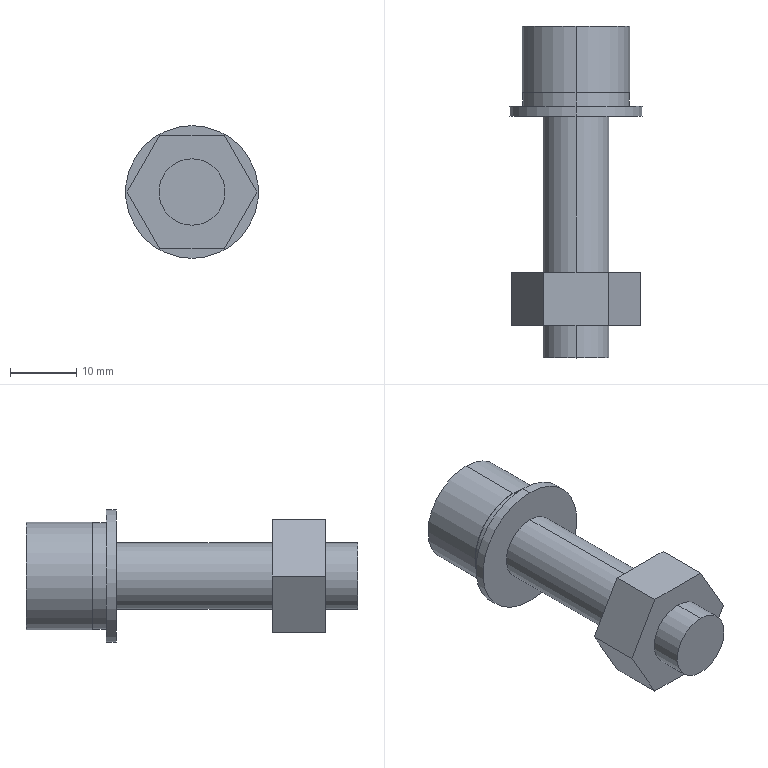Part | SolidWorks | features ICE 4, Revolution 1 | 3 solids | 36 faces | box 20 x 50 x 20 mm | volume 6831 mm3 | plane 22 | cylinder 14 | commonest cylinder face diameters 10 x8 16 x2 16.2 x2 20 x2
STEP:
#1=CARTESIAN_POINT('',(0.,-2.1,5.));
#2=VERTEX_POINT('',#1);
#3=CARTESIAN_POINT('',(0.,-2.1,-5.));
#4=VERTEX_POINT('',#3);
#5=CARTESIAN_POINT('',(0.,-2.1,0.));
#6=DIRECTION('',(0.,-1.,0.));
#7=DIRECTION('',(0.,0.,-1.));
#8=AXIS2_PLACEMENT_3D('',#5,#6,#7);
#9=CIRCLE('',#8,5.);
#10=EDGE_CURVE('',#2,#4,#9,.T.);
#11=ORIENTED_EDGE('',*,*,#10,.T.);
#12=CARTESIAN_POINT('',(0.,0.,-5.));
#13=VERTEX_POINT('',#12);
#14=CARTESIAN_POINT('',(0.,-2.1,-5.));
#15=DIRECTION('',(0.,1.,0.));
#16=VECTOR('',#15,1000.);
#17=LINE('',#14,#16);
#18=EDGE_CURVE('',#4,#13,#17,.T.);
#19=ORIENTED_EDGE('',*,*,#18,.T.);
#20=CARTESIAN_POINT('',(0.,0.,5.));
#21=VERTEX_POINT('',#20);
#22=CARTESIAN_POINT('',(0.,0.,0.));
#23=DIRECTION('',(0.,-1.,0.));
#24=DIRECTION('',(0.,0.,-1.));
#25=AXIS2_PLACEMENT_3D('',#22,#23,#24);
#26=CIRCLE('',#25,5.);
#27=EDGE_CURVE('',#21,#13,#26,.T.);
#28=ORIENTED_EDGE('',*,*,#27,.F.);
#29=CARTESIAN_POINT('',(0.,-2.1,5.));
#30=DIRECTION('',(0.,1.,0.));
#31=VECTOR('',#30,1000.);
#32=LINE('',#29,#31);
#33=EDGE_CURVE('',#2,#21,#32,.T.);
#34=ORIENTED_EDGE('',*,*,#33,.F.);
#35=EDGE_LOOP('',(#11,#19,#28,#34));
#36=FACE_OUTER_BOUND('',#35,.T.);
#37=CARTESIAN_POINT('',(0.,-2.1,0.));
#38=DIRECTION('',(0.,1.,0.));
#39=DIRECTION('',(0.,0.,1.));
#40=AXIS2_PLACEMENT_3D('',#37,#38,#39);
#41=CYLINDRICAL_SURFACE('',#40,5.);
#42=ADVANCED_FACE('',(#36),#41,.F.);
#43=CARTESIAN_POINT('',(0.,-2.1,-8.));
#44=VERTEX_POINT('',#43);
#45=CARTESIAN_POINT('',(0.,-2.1,8.));
#46=VERTEX_POINT('',#45);
#47=CARTESIAN_POINT('',(0.,-2.1,0.));
#48=DIRECTION('',(0.,-1.,0.));
#49=DIRECTION('',(0.,0.,-1.));
#50=AXIS2_PLACEMENT_3D('',#47,#48,#49);
#51=CIRCLE('',#50,8.);
#52=EDGE_CURVE('',#44,#46,#51,.T.);
#53=ORIENTED_EDGE('',*,*,#52,.F.);
#54=CARTESIAN_POINT('',(0.,0.,-8.));
#55=VERTEX_POINT('',#54);
#56=CARTESIAN_POINT('',(0.,-2.1,-8.));
#57=DIRECTION('',(0.,1.,0.));
#58=VECTOR('',#57,1000.);
#59=LINE('',#56,#58);
#60=EDGE_CURVE('',#44,#55,#59,.T.);
#61=ORIENTED_EDGE('',*,*,#60,.T.);
#62=CARTESIAN_POINT('',(0.,0.,8.));
#63=VERTEX_POINT('',#62);
#64=CARTESIAN_POINT('',(0.,0.,0.));
#65=DIRECTION('',(0.,-1.,0.));
#66=DIRECTION('',(0.,0.,-1.));
#67=AXIS2_PLACEMENT_3D('',#64,#65,#66);
#68=CIRCLE('',#67,8.);
#69=EDGE_CURVE('',#55,#63,#68,.T.);
#70=ORIENTED_EDGE('',*,*,#69,.T.);
#71=CARTESIAN_POINT('',(0.,-2.1,8.));
#72=DIRECTION('',(0.,1.,0.));
#73=VECTOR('',#72,1000.);
#74=LINE('',#71,#73);
#75=EDGE_CURVE('',#46,#63,#74,.T.);
#76=ORIENTED_EDGE('',*,*,#75,.F.);
#77=EDGE_LOOP('',(#53,#61,#70,#76));
#78=FACE_OUTER_BOUND('',#77,.T.);
#79=CARTESIAN_POINT('',(0.,-2.1,0.));
#80=DIRECTION('',(0.,1.,0.));
#81=DIRECTION('',(0.,0.,1.));
#82=AXIS2_PLACEMENT_3D('',#79,#80,#81);
#83=CYLINDRICAL_SURFACE('',#82,8.);
#84=ADVANCED_FACE('',(#78),#83,.T.);
#85=CARTESIAN_POINT('',(0.,-2.1,0.));
#86=DIRECTION('',(0.,-1.,0.));
#87=DIRECTION('',(0.,0.,-1.));
#88=AXIS2_PLACEMENT_3D('',#85,#86,#87);
#89=CIRCLE('',#88,8.);
#90=EDGE_CURVE('',#46,#44,#89,.T.);
#91=ORIENTED_EDGE('',*,*,#90,.T.);
#92=ORIENTED_EDGE('',*,*,#52,.T.);
#93=EDGE_LOOP('',(#91,#92));
#94=FACE_OUTER_BOUND('',#93,.T.);
#95=ORIENTED_EDGE('',*,*,#10,.F.);
#96=CARTESIAN_POINT('',(0.,-2.1,0.));
#97=DIRECTION('',(0.,-1.,0.));
#98=DIRECTION('',(0.,0.,-1.));
#99=AXIS2_PLACEMENT_3D('',#96,#97,#98);
#100=CIRCLE('',#99,5.);
#101=EDGE_CURVE('',#4,#2,#100,.T.);
#102=ORIENTED_EDGE('',*,*,#101,.F.);
#103=EDGE_LOOP('',(#95,#102));
#104=FACE_BOUND('',#103,.T.);
#105=CARTESIAN_POINT('',(0.,-2.1,0.));
#106=DIRECTION('',(0.,-1.,0.));
#107=DIRECTION('',(0.,0.,-1.));
#108=AXIS2_PLACEMENT_3D('',#105,#106,#107);
#109=PLANE('',#108);
#110=ADVANCED_FACE('',(#94,#104),#109,.T.);
#111=CARTESIAN_POINT('',(0.,0.,0.));
#112=DIRECTION('',(0.,-1.,0.));
#113=DIRECTION('',(0.,0.,-1.));
#114=AXIS2_PLACEMENT_3D('',#111,#112,#113);
#115=CIRCLE('',#114,8.);
#116=EDGE_CURVE('',#63,#55,#115,.T.);
#117=ORIENTED_EDGE('',*,*,#116,.F.);
#118=ORIENTED_EDGE('',*,*,#69,.F.);
#119=EDGE_LOOP('',(#117,#118));
#120=FACE_OUTER_BOUND('',#119,.T.);
#121=ORIENTED_EDGE('',*,*,#27,.T.);
#122=CARTESIAN_POINT('',(0.,0.,0.));
#123=DIRECTION('',(0.,-1.,0.));
#124=DIRECTION('',(0.,0.,-1.));
#125=AXIS2_PLACEMENT_3D('',#122,#123,#124);
#126=CIRCLE('',#125,5.);
#127=EDGE_CURVE('',#13,#21,#126,.T.);
#128=ORIENTED_EDGE('',*,*,#127,.T.);
#129=EDGE_LOOP('',(#121,#128));
#130=FACE_BOUND('',#129,.T.);
#131=CARTESIAN_POINT('',(0.,0.,0.));
#132=DIRECTION('',(0.,-1.,0.));
#133=DIRECTION('',(0.,0.,-1.));
#134=AXIS2_PLACEMENT_3D('',#131,#132,#133);
#135=PLANE('',#134);
#136=ADVANCED_FACE('',(#120,#130),#135,.F.);
#137=ORIENTED_EDGE('',*,*,#60,.F.);
#138=ORIENTED_EDGE('',*,*,#90,.F.);
#139=ORIENTED_EDGE('',*,*,#75,.T.);
#140=ORIENTED_EDGE('',*,*,#116,.T.);
#141=EDGE_LOOP('',(#137,#138,#139,#140));
#142=FACE_OUTER_BOUND('',#141,.T.);
#143=CARTESIAN_POINT('',(0.,-2.1,0.));
#144=DIRECTION('',(0.,1.,0.));
#145=DIRECTION('',(0.,0.,1.));
#146=AXIS2_PLACEMENT_3D('',#143,#144,#145);
#147=CYLINDRICAL_SURFACE('',#146,8.);
#148=ADVANCED_FACE('',(#142),#147,.T.);
#149=ORIENTED_EDGE('',*,*,#18,.F.);
#150=ORIENTED_EDGE('',*,*,#101,.T.);
#151=ORIENTED_EDGE('',*,*,#33,.T.);
#152=ORIENTED_EDGE('',*,*,#127,.F.);
#153=EDGE_LOOP('',(#149,#150,#151,#152));
#154=FACE_OUTER_BOUND('',#153,.T.);
#155=CARTESIAN_POINT('',(0.,-2.1,0.));
#156=DIRECTION('',(0.,1.,0.));
#157=DIRECTION('',(0.,0.,1.));
#158=AXIS2_PLACEMENT_3D('',#155,#156,#157);
#159=CYLINDRICAL_SURFACE('',#158,5.);
#160=ADVANCED_FACE('',(#154),#159,.F.);
#161=CLOSED_SHELL('',(#42,#84,#110,#136,#148,#160));
#162=MANIFOLD_SOLID_BREP('',#161);
#163=CARTESIAN_POINT('',(0.,-3.6,5.));
#164=VERTEX_POINT('',#163);
#165=CARTESIAN_POINT('',(0.,-3.6,-5.));
#166=VERTEX_POINT('',#165);
#167=CARTESIAN_POINT('',(0.,-3.6,0.));
#168=DIRECTION('',(0.,-1.,0.));
#169=DIRECTION('',(0.,0.,-1.));
#170=AXIS2_PLACEMENT_3D('',#167,#168,#169);
#171=CIRCLE('',#170,5.);
#172=EDGE_CURVE('',#164,#166,#171,.T.);
#173=ORIENTED_EDGE('',*,*,#172,.T.);
#174=CARTESIAN_POINT('',(0.,-2.1,-5.));
#175=VERTEX_POINT('',#174);
#176=CARTESIAN_POINT('',(0.,-3.6,-5.));
#177=DIRECTION('',(0.,1.,0.));
#178=VECTOR('',#177,1000.);
#179=LINE('',#176,#178);
#180=EDGE_CURVE('',#166,#175,#179,.T.);
#181=ORIENTED_EDGE('',*,*,#180,.T.);
#182=CARTESIAN_POINT('',(0.,-2.1,5.));
#183=VERTEX_POINT('',#182);
#184=CARTESIAN_POINT('',(0.,-2.1,0.));
#185=DIRECTION('',(0.,-1.,0.));
#186=DIRECTION('',(0.,0.,-1.));
#187=AXIS2_PLACEMENT_3D('',#184,#185,#186);
#188=CIRCLE('',#187,5.);
#189=EDGE_CURVE('',#183,#175,#188,.T.);
#190=ORIENTED_EDGE('',*,*,#189,.F.);
#191=CARTESIAN_POINT('',(0.,-3.6,5.));
#192=DIRECTION('',(0.,1.,0.));
#193=VECTOR('',#192,1000.);
#194=LINE('',#191,#193);
#195=EDGE_CURVE('',#164,#183,#194,.T.);
#196=ORIENTED_EDGE('',*,*,#195,.F.);
#197=EDGE_LOOP('',(#173,#181,#190,#196));
#198=FACE_OUTER_BOUND('',#197,.T.);
#199=CARTESIAN_POINT('',(0.,-3.6,0.));
#200=DIRECTION('',(0.,1.,0.));
#201=DIRECTION('',(0.,0.,1.));
#202=AXIS2_PLACEMENT_3D('',#199,#200,#201);
#203=CYLINDRICAL_SURFACE('',#202,5.);
#204=ADVANCED_FACE('',(#198),#203,.F.);
#205=CARTESIAN_POINT('',(0.,-3.6,-10.));
#206=VERTEX_POINT('',#205);
#207=CARTESIAN_POINT('',(0.,-3.6,10.));
#208=VERTEX_POINT('',#207);
#209=CARTESIAN_POINT('',(0.,-3.6,0.));
#210=DIRECTION('',(0.,-1.,0.));
#211=DIRECTION('',(0.,0.,-1.));
#212=AXIS2_PLACEMENT_3D('',#209,#210,#211);
#213=CIRCLE('',#212,10.);
#214=EDGE_CURVE('',#206,#208,#213,.T.);
#215=ORIENTED_EDGE('',*,*,#214,.F.);
#216=CARTESIAN_POINT('',(0.,-2.1,-10.));
#217=VERTEX_POINT('',#216);
#218=CARTESIAN_POINT('',(0.,-3.6,-10.));
#219=DIRECTION('',(0.,1.,0.));
#220=VECTOR('',#219,1000.);
#221=LINE('',#218,#220);
#222=EDGE_CURVE('',#206,#217,#221,.T.);
#223=ORIENTED_EDGE('',*,*,#222,.T.);
#224=CARTESIAN_POINT('',(0.,-2.1,10.));
#225=VERTEX_POINT('',#224);
#226=CARTESIAN_POINT('',(0.,-2.1,0.));
#227=DIRECTION('',(0.,-1.,0.));
#228=DIRECTION('',(0.,0.,-1.));
#229=AXIS2_PLACEMENT_3D('',#226,#227,#228);
#230=CIRCLE('',#229,10.);
#231=EDGE_CURVE('',#217,#225,#230,.T.);
#232=ORIENTED_EDGE('',*,*,#231,.T.);
#233=CARTESIAN_POINT('',(0.,-3.6,10.));
#234=DIRECTION('',(0.,1.,0.));
#235=VECTOR('',#234,1000.);
#236=LINE('',#233,#235);
#237=EDGE_CURVE('',#208,#225,#236,.T.);
#238=ORIENTED_EDGE('',*,*,#237,.F.);
#239=EDGE_LOOP('',(#215,#223,#232,#238));
#240=FACE_OUTER_BOUND('',#239,.T.);
#241=CARTESIAN_POINT('',(0.,-3.6,0.));
#242=DIRECTION('',(0.,1.,0.));
#243=DIRECTION('',(0.,0.,1.));
#244=AXIS2_PLACEMENT_3D('',#241,#242,#243);
#245=CYLINDRICAL_SURFACE('',#244,10.);
#246=ADVANCED_FACE('',(#240),#245,.T.);
#247=CARTESIAN_POINT('',(0.,-3.6,0.));
#248=DIRECTION('',(0.,-1.,0.));
#249=DIRECTION('',(0.,0.,-1.));
#250=AXIS2_PLACEMENT_3D('',#247,#248,#249);
#251=CIRCLE('',#250,10.);
#252=EDGE_CURVE('',#208,#206,#251,.T.);
#253=ORIENTED_EDGE('',*,*,#252,.T.);
#254=ORIENTED_EDGE('',*,*,#214,.T.);
#255=EDGE_LOOP('',(#253,#254));
#256=FACE_OUTER_BOUND('',#255,.T.);
#257=ORIENTED_EDGE('',*,*,#172,.F.);
#258=CARTESIAN_POINT('',(0.,-3.6,0.));
#259=DIRECTION('',(0.,-1.,0.));
#260=DIRECTION('',(0.,0.,-1.));
#261=AXIS2_PLACEMENT_3D('',#258,#259,#260);
#262=CIRCLE('',#261,5.);
#263=EDGE_CURVE('',#166,#164,#262,.T.);
#264=ORIENTED_EDGE('',*,*,#263,.F.);
#265=EDGE_LOOP('',(#257,#264));
#266=FACE_BOUND('',#265,.T.);
#267=CARTESIAN_POINT('',(0.,-3.6,0.));
#268=DIRECTION('',(0.,-1.,0.));
#269=DIRECTION('',(0.,0.,-1.));
#270=AXIS2_PLACEMENT_3D('',#267,#268,#269);
#271=PLANE('',#270);
#272=ADVANCED_FACE('',(#256,#266),#271,.T.);
#273=CARTESIAN_POINT('',(0.,-2.1,0.));
#274=DIRECTION('',(0.,-1.,0.));
#275=DIRECTION('',(0.,0.,-1.));
#276=AXIS2_PLACEMENT_3D('',#273,#274,#275);
#277=CIRCLE('',#276,10.);
#278=EDGE_CURVE('',#225,#217,#277,.T.);
#279=ORIENTED_EDGE('',*,*,#278,.F.);
#280=ORIENTED_EDGE('',*,*,#231,.F.);
#281=EDGE_LOOP('',(#279,#280));
#282=FACE_OUTER_BOUND('',#281,.T.);
#283=ORIENTED_EDGE('',*,*,#189,.T.);
#284=CARTESIAN_POINT('',(0.,-2.1,0.));
#285=DIRECTION('',(0.,-1.,0.));
#286=DIRECTION('',(0.,0.,-1.));
#287=AXIS2_PLACEMENT_3D('',#284,#285,#286);
#288=CIRCLE('',#287,5.);
#289=EDGE_CURVE('',#175,#183,#288,.T.);
#290=ORIENTED_EDGE('',*,*,#289,.T.);
#291=EDGE_LOOP('',(#283,#290));
#292=FACE_BOUND('',#291,.T.);
#293=CARTESIAN_POINT('',(0.,-2.1,0.));
#294=DIRECTION('',(0.,-1.,0.));
#295=DIRECTION('',(0.,0.,-1.));
#296=AXIS2_PLACEMENT_3D('',#293,#294,#295);
#297=PLANE('',#296);
#298=ADVANCED_FACE('',(#282,#292),#297,.F.);
#299=ORIENTED_EDGE('',*,*,#222,.F.);
#300=ORIENTED_EDGE('',*,*,#252,.F.);
#301=ORIENTED_EDGE('',*,*,#237,.T.);
#302=ORIENTED_EDGE('',*,*,#278,.T.);
#303=EDGE_LOOP('',(#299,#300,#301,#302));
#304=FACE_OUTER_BOUND('',#303,.T.);
#305=CARTESIAN_POINT('',(0.,-3.6,0.));
#306=DIRECTION('',(0.,1.,0.));
#307=DIRECTION('',(0.,0.,1.));
#308=AXIS2_PLACEMENT_3D('',#305,#306,#307);
#309=CYLINDRICAL_SURFACE('',#308,10.);
#310=ADVANCED_FACE('',(#304),#309,.T.);
#311=ORIENTED_EDGE('',*,*,#180,.F.);
#312=ORIENTED_EDGE('',*,*,#263,.T.);
#313=ORIENTED_EDGE('',*,*,#195,.T.);
#314=ORIENTED_EDGE('',*,*,#289,.F.);
#315=EDGE_LOOP('',(#311,#312,#313,#314));
#316=FACE_OUTER_BOUND('',#315,.T.);
#317=CARTESIAN_POINT('',(0.,-3.6,0.));
#318=DIRECTION('',(0.,1.,0.));
#319=DIRECTION('',(0.,0.,1.));
#320=AXIS2_PLACEMENT_3D('',#317,#318,#319);
#321=CYLINDRICAL_SURFACE('',#320,5.);
#322=ADVANCED_FACE('',(#316),#321,.F.);
#323=CLOSED_SHELL('',(#204,#246,#272,#298,#310,#322));
#324=MANIFOLD_SOLID_BREP('',#323);
#325=CARTESIAN_POINT('',(0.,-40.,5.));
#326=VERTEX_POINT('',#325);
#327=CARTESIAN_POINT('',(0.,-40.,-5.));
#328=VERTEX_POINT('',#327);
#329=CARTESIAN_POINT('',(0.,-40.,0.));
#330=DIRECTION('',(0.,1.,0.));
#331=DIRECTION('',(0.,0.,1.));
#332=AXIS2_PLACEMENT_3D('',#329,#330,#331);
#333=CIRCLE('',#332,5.);
#334=EDGE_CURVE('',#326,#328,#333,.T.);
#335=ORIENTED_EDGE('',*,*,#334,.T.);
#336=CARTESIAN_POINT('',(0.,-35.1,-5.));
#337=VERTEX_POINT('',#336);
#338=CARTESIAN_POINT('',(0.,11.322,-5.));
#339=DIRECTION('',(0.,1.,0.));
#340=VECTOR('',#339,1000.);
#341=LINE('',#338,#340);
#342=EDGE_CURVE('',#328,#337,#341,.T.);
#343=ORIENTED_EDGE('',*,*,#342,.T.);
#344=CARTESIAN_POINT('',(0.,-35.1,5.));
#345=VERTEX_POINT('',#344);
#346=CARTESIAN_POINT('',(0.,-35.1,0.));
#347=DIRECTION('',(0.,1.,0.));
#348=DIRECTION('',(0.,0.,-1.));
#349=AXIS2_PLACEMENT_3D('',#346,#347,#348);
#350=CIRCLE('',#349,5.);
#351=EDGE_CURVE('',#345,#337,#350,.T.);
#352=ORIENTED_EDGE('',*,*,#351,.F.);
#353=CARTESIAN_POINT('',(0.,11.322,5.));
#354=DIRECTION('',(0.,1.,0.));
#355=VECTOR('',#354,1000.);
#356=LINE('',#353,#355);
#357=EDGE_CURVE('',#326,#345,#356,.T.);
#358=ORIENTED_EDGE('',*,*,#357,.F.);
#359=EDGE_LOOP('',(#335,#343,#352,#358));
#360=FACE_OUTER_BOUND('',#359,.T.);
#361=CARTESIAN_POINT('',(0.,11.322,0.));
#362=DIRECTION('',(0.,1.,0.));
#363=DIRECTION('',(0.,0.,1.));
#364=AXIS2_PLACEMENT_3D('',#361,#362,#363);
#365=CYLINDRICAL_SURFACE('',#364,5.);
#366=ADVANCED_FACE('',(#360),#365,.T.);
#367=CARTESIAN_POINT('',(0.,0.,8.1));
#368=VERTEX_POINT('',#367);
#369=CARTESIAN_POINT('',(0.,0.,-8.1));
#370=VERTEX_POINT('',#369);
#371=CARTESIAN_POINT('',(0.,0.,0.));
#372=DIRECTION('',(0.,1.,0.));
#373=DIRECTION('',(0.,0.,1.));
#374=AXIS2_PLACEMENT_3D('',#371,#372,#373);
#375=CIRCLE('',#374,8.1);
#376=EDGE_CURVE('',#368,#370,#375,.T.);
#377=ORIENTED_EDGE('',*,*,#376,.T.);
#378=CARTESIAN_POINT('',(0.,10.,-8.1));
#379=VERTEX_POINT('',#378);
#380=CARTESIAN_POINT('',(0.,11.322,-8.1));
#381=DIRECTION('',(0.,1.,0.));
#382=VECTOR('',#381,1000.);
#383=LINE('',#380,#382);
#384=EDGE_CURVE('',#370,#379,#383,.T.);
#385=ORIENTED_EDGE('',*,*,#384,.T.);
#386=CARTESIAN_POINT('',(0.,10.,8.1));
#387=VERTEX_POINT('',#386);
#388=CARTESIAN_POINT('',(0.,10.,0.));
#389=DIRECTION('',(0.,1.,0.));
#390=DIRECTION('',(0.,0.,1.));
#391=AXIS2_PLACEMENT_3D('',#388,#389,#390);
#392=CIRCLE('',#391,8.1);
#393=EDGE_CURVE('',#387,#379,#392,.T.);
#394=ORIENTED_EDGE('',*,*,#393,.F.);
#395=CARTESIAN_POINT('',(0.,11.322,8.1));
#396=DIRECTION('',(0.,1.,0.));
#397=VECTOR('',#396,1000.);
#398=LINE('',#395,#397);
#399=EDGE_CURVE('',#368,#387,#398,.T.);
#400=ORIENTED_EDGE('',*,*,#399,.F.);
#401=EDGE_LOOP('',(#377,#385,#394,#400));
#402=FACE_OUTER_BOUND('',#401,.T.);
#403=CARTESIAN_POINT('',(0.,11.322,0.));
#404=DIRECTION('',(0.,1.,0.));
#405=DIRECTION('',(0.,0.,1.));
#406=AXIS2_PLACEMENT_3D('',#403,#404,#405);
#407=CYLINDRICAL_SURFACE('',#406,8.1);
#408=ADVANCED_FACE('',(#402),#407,.T.);
#409=CARTESIAN_POINT('',(0.,-27.1,-5.));
#410=VERTEX_POINT('',#409);
#411=CARTESIAN_POINT('',(0.,-27.1,5.));
#412=VERTEX_POINT('',#411);
#413=CARTESIAN_POINT('',(0.,-27.1,0.));
#414=DIRECTION('',(0.,-1.,0.));
#415=DIRECTION('',(0.,0.,-1.));
#416=AXIS2_PLACEMENT_3D('',#413,#414,#415);
#417=CIRCLE('',#416,5.);
#418=EDGE_CURVE('',#410,#412,#417,.T.);
#419=ORIENTED_EDGE('',*,*,#418,.F.);
#420=CARTESIAN_POINT('',(0.,0.,-5.));
#421=VERTEX_POINT('',#420);
#422=CARTESIAN_POINT('',(0.,11.322,-5.));
#423=DIRECTION('',(0.,1.,0.));
#424=VECTOR('',#423,1000.);
#425=LINE('',#422,#424);
#426=EDGE_CURVE('',#410,#421,#425,.T.);
#427=ORIENTED_EDGE('',*,*,#426,.T.);
#428=CARTESIAN_POINT('',(0.,0.,5.));
#429=VERTEX_POINT('',#428);
#430=CARTESIAN_POINT('',(0.,0.,0.));
#431=DIRECTION('',(0.,1.,0.));
#432=DIRECTION('',(0.,0.,1.));
#433=AXIS2_PLACEMENT_3D('',#430,#431,#432);
#434=CIRCLE('',#433,5.);
#435=EDGE_CURVE('',#429,#421,#434,.T.);
#436=ORIENTED_EDGE('',*,*,#435,.F.);
#437=CARTESIAN_POINT('',(0.,11.322,5.));
#438=DIRECTION('',(0.,1.,0.));
#439=VECTOR('',#438,1000.);
#440=LINE('',#437,#439);
#441=EDGE_CURVE('',#412,#429,#440,.T.);
#442=ORIENTED_EDGE('',*,*,#441,.F.);
#443=EDGE_LOOP('',(#419,#427,#436,#442));
#444=FACE_OUTER_BOUND('',#443,.T.);
#445=CARTESIAN_POINT('',(0.,11.322,0.));
#446=DIRECTION('',(0.,1.,0.));
#447=DIRECTION('',(0.,0.,1.));
#448=AXIS2_PLACEMENT_3D('',#445,#446,#447);
#449=CYLINDRICAL_SURFACE('',#448,5.);
#450=ADVANCED_FACE('',(#444),#449,.T.);
#451=ORIENTED_EDGE('',*,*,#426,.F.);
#452=CARTESIAN_POINT('',(0.,-27.1,0.));
#453=DIRECTION('',(0.,-1.,0.));
#454=DIRECTION('',(0.,0.,-1.));
#455=AXIS2_PLACEMENT_3D('',#452,#453,#454);
#456=CIRCLE('',#455,5.);
#457=EDGE_CURVE('',#412,#410,#456,.T.);
#458=ORIENTED_EDGE('',*,*,#457,.F.);
#459=ORIENTED_EDGE('',*,*,#441,.T.);
#460=CARTESIAN_POINT('',(0.,0.,0.));
#461=DIRECTION('',(0.,1.,0.));
#462=DIRECTION('',(0.,0.,1.));
#463=AXIS2_PLACEMENT_3D('',#460,#461,#462);
#464=CIRCLE('',#463,5.);
#465=EDGE_CURVE('',#421,#429,#464,.T.);
#466=ORIENTED_EDGE('',*,*,#465,.F.);
#467=EDGE_LOOP('',(#451,#458,#459,#466));
#468=FACE_OUTER_BOUND('',#467,.T.);
#469=CARTESIAN_POINT('',(0.,11.322,0.));
#470=DIRECTION('',(0.,1.,0.));
#471=DIRECTION('',(0.,0.,1.));
#472=AXIS2_PLACEMENT_3D('',#469,#470,#471);
#473=CYLINDRICAL_SURFACE('',#472,5.);
#474=ADVANCED_FACE('',(#468),#473,.T.);
#475=CARTESIAN_POINT('',(4.,10.,-2.309));
#476=VERTEX_POINT('',#475);
#477=CARTESIAN_POINT('',(0.,10.,-4.619));
#478=VERTEX_POINT('',#477);
#479=CARTESIAN_POINT('',(4.,10.,-2.309));
#480=DIRECTION('',(-0.866,0.,-0.5));
#481=VECTOR('',#480,1000.);
#482=LINE('',#479,#481);
#483=EDGE_CURVE('',#476,#478,#482,.T.);
#484=ORIENTED_EDGE('',*,*,#483,.F.);
#485=CARTESIAN_POINT('',(4.,10.,2.309));
#486=VERTEX_POINT('',#485);
#487=CARTESIAN_POINT('',(4.,10.,2.309));
#488=DIRECTION('',(0.,0.,-1.));
#489=VECTOR('',#488,1000.);
#490=LINE('',#487,#489);
#491=EDGE_CURVE('',#486,#476,#490,.T.);
#492=ORIENTED_EDGE('',*,*,#491,.F.);
#493=CARTESIAN_POINT('',(0.,10.,4.619));
#494=VERTEX_POINT('',#493);
#495=CARTESIAN_POINT('',(0.,10.,4.619));
#496=DIRECTION('',(0.866,0.,-0.5));
#497=VECTOR('',#496,1000.);
#498=LINE('',#495,#497);
#499=EDGE_CURVE('',#494,#486,#498,.T.);
#500=ORIENTED_EDGE('',*,*,#499,.F.);
#501=CARTESIAN_POINT('',(-4.,10.,2.309));
#502=VERTEX_POINT('',#501);
#503=CARTESIAN_POINT('',(-4.,10.,2.309));
#504=DIRECTION('',(0.866,0.,0.5));
#505=VECTOR('',#504,1000.);
#506=LINE('',#503,#505);
#507=EDGE_CURVE('',#502,#494,#506,.T.);
#508=ORIENTED_EDGE('',*,*,#507,.F.);
#509=CARTESIAN_POINT('',(-4.,10.,-2.309));
#510=VERTEX_POINT('',#509);
#511=CARTESIAN_POINT('',(-4.,10.,-2.309));
#512=DIRECTION('',(0.,0.,1.));
#513=VECTOR('',#512,1000.);
#514=LINE('',#511,#513);
#515=EDGE_CURVE('',#510,#502,#514,.T.);
#516=ORIENTED_EDGE('',*,*,#515,.F.);
#517=CARTESIAN_POINT('',(0.,10.,-4.619));
#518=DIRECTION('',(-0.866,0.,0.5));
#519=VECTOR('',#518,1000.);
#520=LINE('',#517,#519);
#521=EDGE_CURVE('',#478,#510,#520,.T.);
#522=ORIENTED_EDGE('',*,*,#521,.F.);
#523=EDGE_LOOP('',(#484,#492,#500,#508,#516,#522));
#524=FACE_BOUND('',#523,.T.);
#525=ORIENTED_EDGE('',*,*,#393,.T.);
#526=CARTESIAN_POINT('',(0.,10.,0.));
#527=DIRECTION('',(0.,1.,0.));
#528=DIRECTION('',(0.,0.,1.));
#529=AXIS2_PLACEMENT_3D('',#526,#527,#528);
#530=CIRCLE('',#529,8.1);
#531=EDGE_CURVE('',#379,#387,#530,.T.);
#532=ORIENTED_EDGE('',*,*,#531,.T.);
#533=EDGE_LOOP('',(#525,#532));
#534=FACE_OUTER_BOUND('',#533,.T.);
#535=CARTESIAN_POINT('',(0.,10.,0.));
#536=DIRECTION('',(0.,1.,0.));
#537=DIRECTION('',(0.,0.,1.));
#538=AXIS2_PLACEMENT_3D('',#535,#536,#537);
#539=PLANE('',#538);
#540=ADVANCED_FACE('',(#524,#534),#539,.T.);
#541=ORIENTED_EDGE('',*,*,#384,.F.);
#542=CARTESIAN_POINT('',(0.,0.,0.));
#543=DIRECTION('',(0.,1.,0.));
#544=DIRECTION('',(0.,0.,1.));
#545=AXIS2_PLACEMENT_3D('',#542,#543,#544);
#546=CIRCLE('',#545,8.1);
#547=EDGE_CURVE('',#370,#368,#546,.T.);
#548=ORIENTED_EDGE('',*,*,#547,.T.);
#549=ORIENTED_EDGE('',*,*,#399,.T.);
#550=ORIENTED_EDGE('',*,*,#531,.F.);
#551=EDGE_LOOP('',(#541,#548,#549,#550));
#552=FACE_OUTER_BOUND('',#551,.T.);
#553=CARTESIAN_POINT('',(0.,11.322,0.));
#554=DIRECTION('',(0.,1.,0.));
#555=DIRECTION('',(0.,0.,1.));
#556=AXIS2_PLACEMENT_3D('',#553,#554,#555);
#557=CYLINDRICAL_SURFACE('',#556,8.1);
#558=ADVANCED_FACE('',(#552),#557,.T.);
#559=ORIENTED_EDGE('',*,*,#435,.T.);
#560=ORIENTED_EDGE('',*,*,#465,.T.);
#561=EDGE_LOOP('',(#559,#560));
#562=FACE_BOUND('',#561,.T.);
#563=ORIENTED_EDGE('',*,*,#376,.F.);
#564=ORIENTED_EDGE('',*,*,#547,.F.);
#565=EDGE_LOOP('',(#563,#564));
#566=FACE_OUTER_BOUND('',#565,.T.);
#567=CARTESIAN_POINT('',(-8.1,0.,0.));
#568=DIRECTION('',(0.,-1.,0.));
#569=DIRECTION('',(0.,0.,-1.));
#570=AXIS2_PLACEMENT_3D('',#567,#568,#569);
#571=PLANE('',#570);
#572=ADVANCED_FACE('',(#562,#566),#571,.T.);
#573=ORIENTED_EDGE('',*,*,#483,.T.);
#574=CARTESIAN_POINT('',(0.,4.,-4.619));
#575=VERTEX_POINT('',#574);
#576=CARTESIAN_POINT('',(0.,4.,-4.619));
#577=DIRECTION('',(0.,1.,0.));
#578=VECTOR('',#577,1000.);
#579=LINE('',#576,#578);
#580=EDGE_CURVE('',#575,#478,#579,.T.);
#581=ORIENTED_EDGE('',*,*,#580,.F.);
#582=CARTESIAN_POINT('',(4.,4.,-2.309));
#583=VERTEX_POINT('',#582);
#584=CARTESIAN_POINT('',(4.,4.,-2.309));
#585=DIRECTION('',(-0.866,0.,-0.5));
#586=VECTOR('',#585,1000.);
#587=LINE('',#584,#586);
#588=EDGE_CURVE('',#583,#575,#587,.T.);
#589=ORIENTED_EDGE('',*,*,#588,.F.);
#590=CARTESIAN_POINT('',(4.,4.,-2.309));
#591=DIRECTION('',(0.,1.,0.));
#592=VECTOR('',#591,1000.);
#593=LINE('',#590,#592);
#594=EDGE_CURVE('',#583,#476,#593,.T.);
#595=ORIENTED_EDGE('',*,*,#594,.T.);
#596=EDGE_LOOP('',(#573,#581,#589,#595));
#597=FACE_OUTER_BOUND('',#596,.T.);
#598=CARTESIAN_POINT('',(4.,4.,-2.309));
#599=DIRECTION('',(0.5,0.,-0.866));
#600=DIRECTION('',(-0.866,0.,-0.5));
#601=AXIS2_PLACEMENT_3D('',#598,#599,#600);
#602=PLANE('',#601);
#603=ADVANCED_FACE('',(#597),#602,.F.);
#604=ORIENTED_EDGE('',*,*,#491,.T.);
#605=ORIENTED_EDGE('',*,*,#594,.F.);
#606=CARTESIAN_POINT('',(4.,4.,2.309));
#607=VERTEX_POINT('',#606);
#608=CARTESIAN_POINT('',(4.,4.,2.309));
#609=DIRECTION('',(0.,0.,-1.));
#610=VECTOR('',#609,1000.);
#611=LINE('',#608,#610);
#612=EDGE_CURVE('',#607,#583,#611,.T.);
#613=ORIENTED_EDGE('',*,*,#612,.F.);
#614=CARTESIAN_POINT('',(4.,4.,2.309));
#615=DIRECTION('',(0.,1.,0.));
#616=VECTOR('',#615,1000.);
#617=LINE('',#614,#616);
#618=EDGE_CURVE('',#607,#486,#617,.T.);
#619=ORIENTED_EDGE('',*,*,#618,.T.);
#620=EDGE_LOOP('',(#604,#605,#613,#619));
#621=FACE_OUTER_BOUND('',#620,.T.);
#622=CARTESIAN_POINT('',(4.,4.,2.309));
#623=DIRECTION('',(1.,0.,0.));
#624=DIRECTION('',(0.,0.,-1.));
#625=AXIS2_PLACEMENT_3D('',#622,#623,#624);
#626=PLANE('',#625);
#627=ADVANCED_FACE('',(#621),#626,.F.);
#628=ORIENTED_EDGE('',*,*,#499,.T.);
#629=ORIENTED_EDGE('',*,*,#618,.F.);
#630=CARTESIAN_POINT('',(0.,4.,4.619));
#631=VERTEX_POINT('',#630);
#632=CARTESIAN_POINT('',(0.,4.,4.619));
#633=DIRECTION('',(0.866,0.,-0.5));
#634=VECTOR('',#633,1000.);
#635=LINE('',#632,#634);
#636=EDGE_CURVE('',#631,#607,#635,.T.);
#637=ORIENTED_EDGE('',*,*,#636,.F.);
#638=CARTESIAN_POINT('',(0.,4.,4.619));
#639=DIRECTION('',(0.,1.,0.));
#640=VECTOR('',#639,1000.);
#641=LINE('',#638,#640);
#642=EDGE_CURVE('',#631,#494,#641,.T.);
#643=ORIENTED_EDGE('',*,*,#642,.T.);
#644=EDGE_LOOP('',(#628,#629,#637,#643));
#645=FACE_OUTER_BOUND('',#644,.T.);
#646=CARTESIAN_POINT('',(0.,4.,4.619));
#647=DIRECTION('',(0.5,0.,0.866));
#648=DIRECTION('',(0.866,0.,-0.5));
#649=AXIS2_PLACEMENT_3D('',#646,#647,#648);
#650=PLANE('',#649);
#651=ADVANCED_FACE('',(#645),#650,.F.);
#652=ORIENTED_EDGE('',*,*,#507,.T.);
#653=ORIENTED_EDGE('',*,*,#642,.F.);
#654=CARTESIAN_POINT('',(-4.,4.,2.309));
#655=VERTEX_POINT('',#654);
#656=CARTESIAN_POINT('',(-4.,4.,2.309));
#657=DIRECTION('',(0.866,0.,0.5));
#658=VECTOR('',#657,1000.);
#659=LINE('',#656,#658);
#660=EDGE_CURVE('',#655,#631,#659,.T.);
#661=ORIENTED_EDGE('',*,*,#660,.F.);
#662=CARTESIAN_POINT('',(-4.,4.,2.309));
#663=DIRECTION('',(0.,1.,0.));
#664=VECTOR('',#663,1000.);
#665=LINE('',#662,#664);
#666=EDGE_CURVE('',#655,#502,#665,.T.);
#667=ORIENTED_EDGE('',*,*,#666,.T.);
#668=EDGE_LOOP('',(#652,#653,#661,#667));
#669=FACE_OUTER_BOUND('',#668,.T.);
#670=CARTESIAN_POINT('',(-4.,4.,2.309));
#671=DIRECTION('',(-0.5,0.,0.866));
#672=DIRECTION('',(0.866,0.,0.5));
#673=AXIS2_PLACEMENT_3D('',#670,#671,#672);
#674=PLANE('',#673);
#675=ADVANCED_FACE('',(#669),#674,.F.);
#676=ORIENTED_EDGE('',*,*,#515,.T.);
#677=ORIENTED_EDGE('',*,*,#666,.F.);
#678=CARTESIAN_POINT('',(-4.,4.,-2.309));
#679=VERTEX_POINT('',#678);
#680=CARTESIAN_POINT('',(-4.,4.,-2.309));
#681=DIRECTION('',(0.,0.,1.));
#682=VECTOR('',#681,1000.);
#683=LINE('',#680,#682);
#684=EDGE_CURVE('',#679,#655,#683,.T.);
#685=ORIENTED_EDGE('',*,*,#684,.F.);
#686=CARTESIAN_POINT('',(-4.,4.,-2.309));
#687=DIRECTION('',(0.,1.,0.));
#688=VECTOR('',#687,1000.);
#689=LINE('',#686,#688);
#690=EDGE_CURVE('',#679,#510,#689,.T.);
#691=ORIENTED_EDGE('',*,*,#690,.T.);
#692=EDGE_LOOP('',(#676,#677,#685,#691));
#693=FACE_OUTER_BOUND('',#692,.T.);
#694=CARTESIAN_POINT('',(-4.,4.,-2.309));
#695=DIRECTION('',(-1.,0.,0.));
#696=DIRECTION('',(0.,0.,1.));
#697=AXIS2_PLACEMENT_3D('',#694,#695,#696);
#698=PLANE('',#697);
#699=ADVANCED_FACE('',(#693),#698,.F.);
#700=ORIENTED_EDGE('',*,*,#521,.T.);
#701=ORIENTED_EDGE('',*,*,#690,.F.);
#702=CARTESIAN_POINT('',(0.,4.,-4.619));
#703=DIRECTION('',(-0.866,0.,0.5));
#704=VECTOR('',#703,1000.);
#705=LINE('',#702,#704);
#706=EDGE_CURVE('',#575,#679,#705,.T.);
#707=ORIENTED_EDGE('',*,*,#706,.F.);
#708=ORIENTED_EDGE('',*,*,#580,.T.);
#709=EDGE_LOOP('',(#700,#701,#707,#708));
#710=FACE_OUTER_BOUND('',#709,.T.);
#711=CARTESIAN_POINT('',(0.,4.,-4.619));
#712=DIRECTION('',(-0.5,0.,-0.866));
#713=DIRECTION('',(-0.866,0.,0.5));
#714=AXIS2_PLACEMENT_3D('',#711,#712,#713);
#715=PLANE('',#714);
#716=ADVANCED_FACE('',(#710),#715,.F.);
#717=ORIENTED_EDGE('',*,*,#588,.T.);
#718=ORIENTED_EDGE('',*,*,#706,.T.);
#719=ORIENTED_EDGE('',*,*,#684,.T.);
#720=ORIENTED_EDGE('',*,*,#660,.T.);
#721=ORIENTED_EDGE('',*,*,#636,.T.);
#722=ORIENTED_EDGE('',*,*,#612,.T.);
#723=EDGE_LOOP('',(#717,#718,#719,#720,#721,#722));
#724=FACE_OUTER_BOUND('',#723,.T.);
#725=CARTESIAN_POINT('',(0.,4.,0.));
#726=DIRECTION('',(0.,1.,0.));
#727=DIRECTION('',(0.,0.,1.));
#728=AXIS2_PLACEMENT_3D('',#725,#726,#727);
#729=PLANE('',#728);
#730=ADVANCED_FACE('',(#724),#729,.T.);
#731=CARTESIAN_POINT('',(4.879,-35.1,-8.45));
#732=VERTEX_POINT('',#731);
#733=CARTESIAN_POINT('',(9.757,-35.1,0.));
#734=VERTEX_POINT('',#733);
#735=CARTESIAN_POINT('',(4.879,-35.1,-8.45));
#736=DIRECTION('',(0.5,0.,0.866));
#737=VECTOR('',#736,1000.);
#738=LINE('',#735,#737);
#739=EDGE_CURVE('',#732,#734,#738,.T.);
#740=ORIENTED_EDGE('',*,*,#739,.T.);
#741=CARTESIAN_POINT('',(4.879,-35.1,8.45));
#742=VERTEX_POINT('',#741);
#743=CARTESIAN_POINT('',(9.757,-35.1,0.));
#744=DIRECTION('',(-0.5,0.,0.866));
#745=VECTOR('',#744,1000.);
#746=LINE('',#743,#745);
#747=EDGE_CURVE('',#734,#742,#746,.T.);
#748=ORIENTED_EDGE('',*,*,#747,.T.);
#749=CARTESIAN_POINT('',(-4.879,-35.1,8.45));
#750=VERTEX_POINT('',#749);
#751=CARTESIAN_POINT('',(4.879,-35.1,8.45));
#752=DIRECTION('',(-1.,0.,0.));
#753=VECTOR('',#752,1000.);
#754=LINE('',#751,#753);
#755=EDGE_CURVE('',#742,#750,#754,.T.);
#756=ORIENTED_EDGE('',*,*,#755,.T.);
#757=CARTESIAN_POINT('',(-9.757,-35.1,0.));
#758=VERTEX_POINT('',#757);
#759=CARTESIAN_POINT('',(-4.879,-35.1,8.45));
#760=DIRECTION('',(-0.5,0.,-0.866));
#761=VECTOR('',#760,1000.);
#762=LINE('',#759,#761);
#763=EDGE_CURVE('',#750,#758,#762,.T.);
#764=ORIENTED_EDGE('',*,*,#763,.T.);
#765=CARTESIAN_POINT('',(-4.879,-35.1,-8.45));
#766=VERTEX_POINT('',#765);
#767=CARTESIAN_POINT('',(-9.757,-35.1,0.));
#768=DIRECTION('',(0.5,0.,-0.866));
#769=VECTOR('',#768,1000.);
#770=LINE('',#767,#769);
#771=EDGE_CURVE('',#758,#766,#770,.T.);
#772=ORIENTED_EDGE('',*,*,#771,.T.);
#773=CARTESIAN_POINT('',(-4.879,-35.1,-8.45));
#774=DIRECTION('',(1.,0.,0.));
#775=VECTOR('',#774,1000.);
#776=LINE('',#773,#775);
#777=EDGE_CURVE('',#766,#732,#776,.T.);
#778=ORIENTED_EDGE('',*,*,#777,.T.);
#779=EDGE_LOOP('',(#740,#748,#756,#764,#772,#778));
#780=FACE_OUTER_BOUND('',#779,.T.);
#781=ORIENTED_EDGE('',*,*,#351,.T.);
#782=CARTESIAN_POINT('',(0.,-35.1,0.));
#783=DIRECTION('',(0.,1.,0.));
#784=DIRECTION('',(0.,0.,-1.));
#785=AXIS2_PLACEMENT_3D('',#782,#783,#784);
#786=CIRCLE('',#785,5.);
#787=EDGE_CURVE('',#337,#345,#786,.T.);
#788=ORIENTED_EDGE('',*,*,#787,.T.);
#789=EDGE_LOOP('',(#781,#788));
#790=FACE_BOUND('',#789,.T.);
#791=CARTESIAN_POINT('',(0.,-35.1,0.));
#792=DIRECTION('',(0.,-1.,0.));
#793=DIRECTION('',(0.,0.,-1.));
#794=AXIS2_PLACEMENT_3D('',#791,#792,#793);
#795=PLANE('',#794);
#796=ADVANCED_FACE('',(#780,#790),#795,.T.);
#797=CARTESIAN_POINT('',(4.879,-27.1,-8.45));
#798=VERTEX_POINT('',#797);
#799=CARTESIAN_POINT('',(9.757,-27.1,0.));
#800=VERTEX_POINT('',#799);
#801=CARTESIAN_POINT('',(4.879,-27.1,-8.45));
#802=DIRECTION('',(0.5,0.,0.866));
#803=VECTOR('',#802,1000.);
#804=LINE('',#801,#803);
#805=EDGE_CURVE('',#798,#800,#804,.T.);
#806=ORIENTED_EDGE('',*,*,#805,.F.);
#807=CARTESIAN_POINT('',(-4.879,-27.1,-8.45));
#808=VERTEX_POINT('',#807);
#809=CARTESIAN_POINT('',(-4.879,-27.1,-8.45));
#810=DIRECTION('',(1.,0.,0.));
#811=VECTOR('',#810,1000.);
#812=LINE('',#809,#811);
#813=EDGE_CURVE('',#808,#798,#812,.T.);
#814=ORIENTED_EDGE('',*,*,#813,.F.);
#815=CARTESIAN_POINT('',(-9.757,-27.1,0.));
#816=VERTEX_POINT('',#815);
#817=CARTESIAN_POINT('',(-9.757,-27.1,0.));
#818=DIRECTION('',(0.5,0.,-0.866));
#819=VECTOR('',#818,1000.);
#820=LINE('',#817,#819);
#821=EDGE_CURVE('',#816,#808,#820,.T.);
#822=ORIENTED_EDGE('',*,*,#821,.F.);
#823=CARTESIAN_POINT('',(-4.879,-27.1,8.45));
#824=VERTEX_POINT('',#823);
#825=CARTESIAN_POINT('',(-4.879,-27.1,8.45));
#826=DIRECTION('',(-0.5,0.,-0.866));
#827=VECTOR('',#826,1000.);
#828=LINE('',#825,#827);
#829=EDGE_CURVE('',#824,#816,#828,.T.);
#830=ORIENTED_EDGE('',*,*,#829,.F.);
#831=CARTESIAN_POINT('',(4.879,-27.1,8.45));
#832=VERTEX_POINT('',#831);
#833=CARTESIAN_POINT('',(4.879,-27.1,8.45));
#834=DIRECTION('',(-1.,0.,0.));
#835=VECTOR('',#834,1000.);
#836=LINE('',#833,#835);
#837=EDGE_CURVE('',#832,#824,#836,.T.);
#838=ORIENTED_EDGE('',*,*,#837,.F.);
#839=CARTESIAN_POINT('',(9.757,-27.1,0.));
#840=DIRECTION('',(-0.5,0.,0.866));
#841=VECTOR('',#840,1000.);
#842=LINE('',#839,#841);
#843=EDGE_CURVE('',#800,#832,#842,.T.);
#844=ORIENTED_EDGE('',*,*,#843,.F.);
#845=EDGE_LOOP('',(#806,#814,#822,#830,#838,#844));
#846=FACE_OUTER_BOUND('',#845,.T.);
#847=ORIENTED_EDGE('',*,*,#457,.T.);
#848=ORIENTED_EDGE('',*,*,#418,.T.);
#849=EDGE_LOOP('',(#847,#848));
#850=FACE_BOUND('',#849,.T.);
#851=CARTESIAN_POINT('',(0.,-27.1,0.));
#852=DIRECTION('',(0.,-1.,0.));
#853=DIRECTION('',(0.,0.,-1.));
#854=AXIS2_PLACEMENT_3D('',#851,#852,#853);
#855=PLANE('',#854);
#856=ADVANCED_FACE('',(#846,#850),#855,.F.);
#857=ORIENTED_EDGE('',*,*,#805,.T.);
#858=CARTESIAN_POINT('',(9.757,-35.1,0.));
#859=DIRECTION('',(0.,1.,0.));
#860=VECTOR('',#859,1000.);
#861=LINE('',#858,#860);
#862=EDGE_CURVE('',#734,#800,#861,.T.);
#863=ORIENTED_EDGE('',*,*,#862,.F.);
#864=ORIENTED_EDGE('',*,*,#739,.F.);
#865=CARTESIAN_POINT('',(4.879,-35.1,-8.45));
#866=DIRECTION('',(0.,1.,0.));
#867=VECTOR('',#866,1000.);
#868=LINE('',#865,#867);
#869=EDGE_CURVE('',#732,#798,#868,.T.);
#870=ORIENTED_EDGE('',*,*,#869,.T.);
#871=EDGE_LOOP('',(#857,#863,#864,#870));
#872=FACE_OUTER_BOUND('',#871,.T.);
#873=CARTESIAN_POINT('',(4.879,-35.1,-8.45));
#874=DIRECTION('',(-0.866,0.,0.5));
#875=DIRECTION('',(0.5,0.,0.866));
#876=AXIS2_PLACEMENT_3D('',#873,#874,#875);
#877=PLANE('',#876);
#878=ADVANCED_FACE('',(#872),#877,.F.);
#879=ORIENTED_EDGE('',*,*,#843,.T.);
#880=CARTESIAN_POINT('',(4.879,-35.1,8.45));
#881=DIRECTION('',(0.,1.,0.));
#882=VECTOR('',#881,1000.);
#883=LINE('',#880,#882);
#884=EDGE_CURVE('',#742,#832,#883,.T.);
#885=ORIENTED_EDGE('',*,*,#884,.F.);
#886=ORIENTED_EDGE('',*,*,#747,.F.);
#887=ORIENTED_EDGE('',*,*,#862,.T.);
#888=EDGE_LOOP('',(#879,#885,#886,#887));
#889=FACE_OUTER_BOUND('',#888,.T.);
#890=CARTESIAN_POINT('',(9.757,-35.1,0.));
#891=DIRECTION('',(-0.866,0.,-0.5));
#892=DIRECTION('',(-0.5,0.,0.866));
#893=AXIS2_PLACEMENT_3D('',#890,#891,#892);
#894=PLANE('',#893);
#895=ADVANCED_FACE('',(#889),#894,.F.);
#896=ORIENTED_EDGE('',*,*,#837,.T.);
#897=CARTESIAN_POINT('',(-4.879,-35.1,8.45));
#898=DIRECTION('',(0.,1.,0.));
#899=VECTOR('',#898,1000.);
#900=LINE('',#897,#899);
#901=EDGE_CURVE('',#750,#824,#900,.T.);
#902=ORIENTED_EDGE('',*,*,#901,.F.);
#903=ORIENTED_EDGE('',*,*,#755,.F.);
#904=ORIENTED_EDGE('',*,*,#884,.T.);
#905=EDGE_LOOP('',(#896,#902,#903,#904));
#906=FACE_OUTER_BOUND('',#905,.T.);
#907=CARTESIAN_POINT('',(4.879,-35.1,8.45));
#908=DIRECTION('',(0.,0.,-1.));
#909=DIRECTION('',(-1.,0.,0.));
#910=AXIS2_PLACEMENT_3D('',#907,#908,#909);
#911=PLANE('',#910);
#912=ADVANCED_FACE('',(#906),#911,.F.);
#913=ORIENTED_EDGE('',*,*,#829,.T.);
#914=CARTESIAN_POINT('',(-9.757,-35.1,0.));
#915=DIRECTION('',(0.,1.,0.));
#916=VECTOR('',#915,1000.);
#917=LINE('',#914,#916);
#918=EDGE_CURVE('',#758,#816,#917,.T.);
#919=ORIENTED_EDGE('',*,*,#918,.F.);
#920=ORIENTED_EDGE('',*,*,#763,.F.);
#921=ORIENTED_EDGE('',*,*,#901,.T.);
#922=EDGE_LOOP('',(#913,#919,#920,#921));
#923=FACE_OUTER_BOUND('',#922,.T.);
#924=CARTESIAN_POINT('',(-4.879,-35.1,8.45));
#925=DIRECTION('',(0.866,0.,-0.5));
#926=DIRECTION('',(-0.5,0.,-0.866));
#927=AXIS2_PLACEMENT_3D('',#924,#925,#926);
#928=PLANE('',#927);
#929=ADVANCED_FACE('',(#923),#928,.F.);
#930=ORIENTED_EDGE('',*,*,#821,.T.);
#931=CARTESIAN_POINT('',(-4.879,-35.1,-8.45));
#932=DIRECTION('',(0.,1.,0.));
#933=VECTOR('',#932,1000.);
#934=LINE('',#931,#933);
#935=EDGE_CURVE('',#766,#808,#934,.T.);
#936=ORIENTED_EDGE('',*,*,#935,.F.);
#937=ORIENTED_EDGE('',*,*,#771,.F.);
#938=ORIENTED_EDGE('',*,*,#918,.T.);
#939=EDGE_LOOP('',(#930,#936,#937,#938));
#940=FACE_OUTER_BOUND('',#939,.T.);
#941=CARTESIAN_POINT('',(-9.757,-35.1,0.));
#942=DIRECTION('',(0.866,0.,0.5));
#943=DIRECTION('',(0.5,0.,-0.866));
#944=AXIS2_PLACEMENT_3D('',#941,#942,#943);
#945=PLANE('',#944);
#946=ADVANCED_FACE('',(#940),#945,.F.);
#947=ORIENTED_EDGE('',*,*,#813,.T.);
#948=ORIENTED_EDGE('',*,*,#869,.F.);
#949=ORIENTED_EDGE('',*,*,#777,.F.);
#950=ORIENTED_EDGE('',*,*,#935,.T.);
#951=EDGE_LOOP('',(#947,#948,#949,#950));
#952=FACE_OUTER_BOUND('',#951,.T.);
#953=CARTESIAN_POINT('',(-4.879,-35.1,-8.45));
#954=DIRECTION('',(0.,0.,1.));
#955=DIRECTION('',(1.,0.,0.));
#956=AXIS2_PLACEMENT_3D('',#953,#954,#955);
#957=PLANE('',#956);
#958=ADVANCED_FACE('',(#952),#957,.F.);
#959=ORIENTED_EDGE('',*,*,#334,.F.);
#960=CARTESIAN_POINT('',(0.,-40.,0.));
#961=DIRECTION('',(0.,1.,0.));
#962=DIRECTION('',(0.,0.,1.));
#963=AXIS2_PLACEMENT_3D('',#960,#961,#962);
#964=CIRCLE('',#963,5.);
#965=EDGE_CURVE('',#328,#326,#964,.T.);
#966=ORIENTED_EDGE('',*,*,#965,.F.);
#967=EDGE_LOOP('',(#959,#966));
#968=FACE_OUTER_BOUND('',#967,.T.);
#969=CARTESIAN_POINT('',(-5.,-40.,0.));
#970=DIRECTION('',(0.,-1.,0.));
#971=DIRECTION('',(0.,0.,-1.));
#972=AXIS2_PLACEMENT_3D('',#969,#970,#971);
#973=PLANE('',#972);
#974=ADVANCED_FACE('',(#968),#973,.T.);
#975=ORIENTED_EDGE('',*,*,#342,.F.);
#976=ORIENTED_EDGE('',*,*,#965,.T.);
#977=ORIENTED_EDGE('',*,*,#357,.T.);
#978=ORIENTED_EDGE('',*,*,#787,.F.);
#979=EDGE_LOOP('',(#975,#976,#977,#978));
#980=FACE_OUTER_BOUND('',#979,.T.);
#981=CARTESIAN_POINT('',(0.,11.322,0.));
#982=DIRECTION('',(0.,1.,0.));
#983=DIRECTION('',(0.,0.,1.));
#984=AXIS2_PLACEMENT_3D('',#981,#982,#983);
#985=CYLINDRICAL_SURFACE('',#984,5.);
#986=ADVANCED_FACE('',(#980),#985,.T.);
#987=CLOSED_SHELL('',(#366,#408,#450,#474,#540,#558,#572,#603,#627,#651,#675,#699,#716,#730,#796,#856,#878,#895,#912,#929,#946,#958,#974,#986));
#988=MANIFOLD_SOLID_BREP('',#987);
#989=CARTESIAN_POINT('',(0.,0.,0.));
#990=DIRECTION('',(0.,0.,1.));
#991=DIRECTION('',(1.,0.,0.));
#992=AXIS2_PLACEMENT_3D('',#989,#990,#991);
#993=(LENGTH_UNIT()NAMED_UNIT(*)SI_UNIT(.MILLI.,.METRE.));
#994=UNCERTAINTY_MEASURE_WITH_UNIT(LENGTH_MEASURE(0.00001),#993,'','');
#995=(NAMED_UNIT(*)PLANE_ANGLE_UNIT()SI_UNIT($,.RADIAN.));
#996=(NAMED_UNIT(*)SI_UNIT($,.STERADIAN.)SOLID_ANGLE_UNIT());
#997=(GEOMETRIC_REPRESENTATION_CONTEXT(3)GLOBAL_UNCERTAINTY_ASSIGNED_CONTEXT((#994))GLOBAL_UNIT_ASSIGNED_CONTEXT((#993,#995,#996))REPRESENTATION_CONTEXT('',''));
#998=ADVANCED_BREP_SHAPE_REPRESENTATION('',(#162,#324,#988,#992),#997);